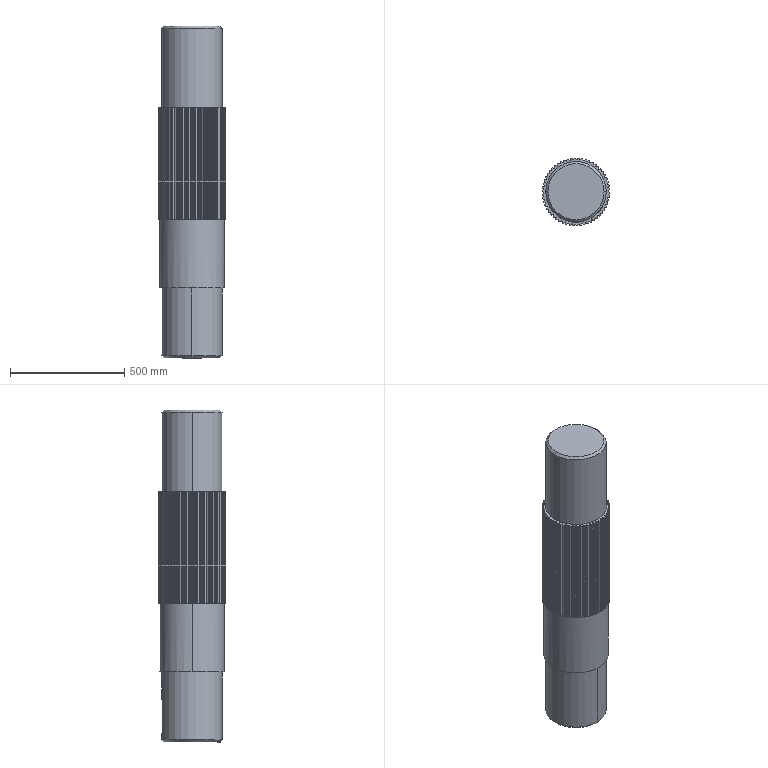Part | SolidWorks | features ICE 5, 3DProfileFeature 1, Chamfer 1, CirPattern 1, Extrusion 1, Fillet 1 | 1 solid | 387 faces | box 294.723 x 294.709 x 1450 mm | volume 87344155 mm3 | cylinder 201 | spline 118 | plane 64 | cone 4 | commonest cylinder face diameters 4 x136 295 x58 265 x5 282.5 x2